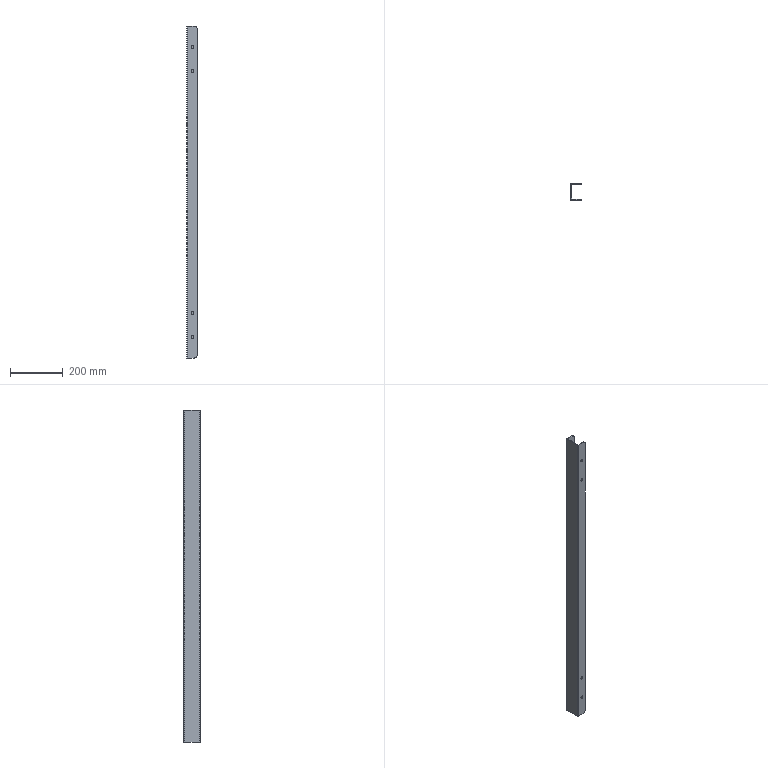Part | SolidWorks | features ICE 2, Cut 1, Fillet 1, FlatPattern 1, SMBaseFlange 1, SheetMetal 1 | 1 solid | 63 faces | box 40 x 62 x 1260 mm | volume 502102 mm3 | cylinder 35 | plane 28 | commonest cylinder face diameters 10 x15 11 x8 12.8 x4 24 x4 0.4 x2 6.4 x2